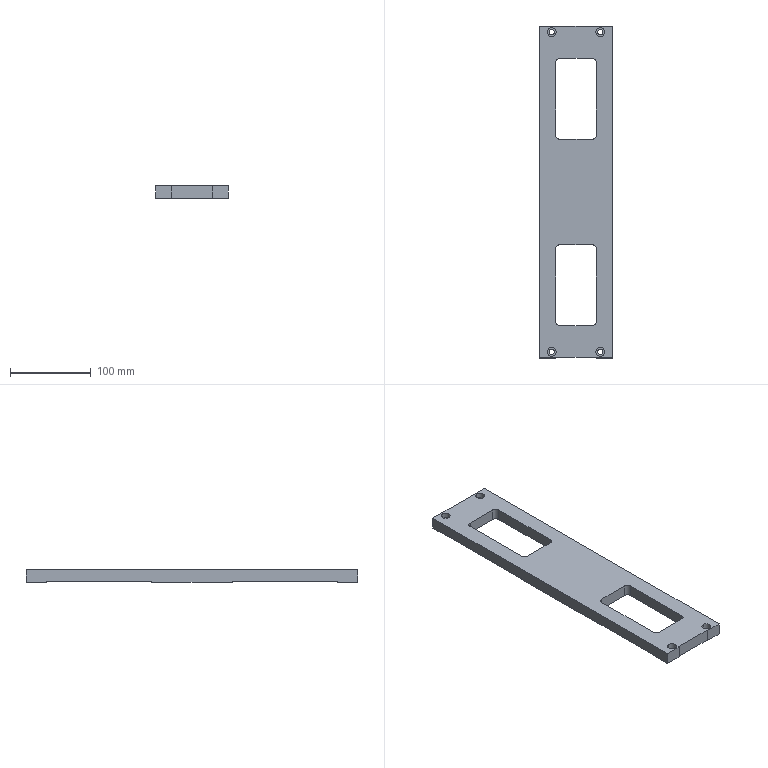NC program | NX | posted with a generic post | part box 90 x 410 x 15 mm
Lines 1 to 55 of 4348:
N10 G17 G21 G94 G90
(DRILLING , TOOL : D6A45)
N12 T07 M6
N14 G54
N16 G17 G0 G90 X197.5 Y30. S5000 M3
N18 G43 Z30. H7
N20 G94 G81 G98 Z-1. F250. R3.
N22 Y0.
N24 Y-30.
N26 X38.5 Y-25.
N28 Y0.
N30 Y25.
N32 Y39.5
N34 X-38.5
N36 Y25.
N38 Y0.
N40 Y-25.
N42 X-197.5 Y-30.
N44 X-198.5 Y0.
N46 X-197.5 Y30.
N48 G80
N50 G0 X-197.5 Y30. Z30.
N52 M5
(DRILLING_COPY , TOOL : 6.6ZT)
N54 T16 M6
N56 G54
N58 G17 G0 G90 X-197.5 Y30. S2000 M3
N60 G43 Z30. H16
N62 G94 G83 G98 Z-16.983 F200. Q2. R3.
N64 Y-30.
N66 X197.5
N68 Y30.
N70 G80
N72 G0 X197.5 Y30. Z30.
N74 M5
(DRILLING_COPY_COPY , TOOL : 3.3ZT)
N76 T13 M6
N78 G54
N80 G17 G0 G90 X-38.5 Y-25. S2000 M3
N82 G43 Z30. H13
N84 G94 G83 G98 Z-11.091 F200. Q2. R3.
N86 Y25.
N88 X38.5
N90 Y-25.
N92 G80
N94 G0 X38.5 Y-25. Z30.
N96 M5